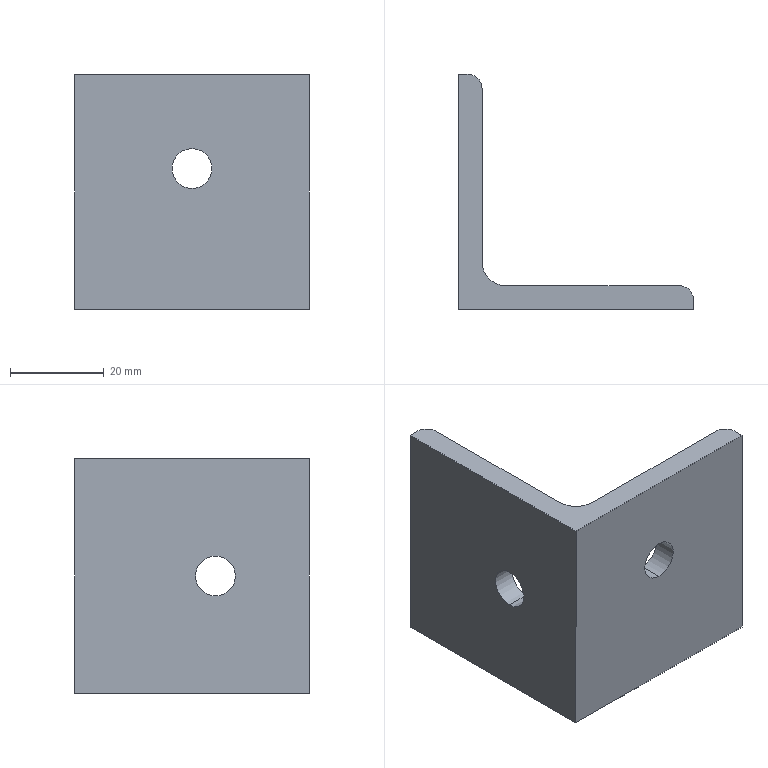Part | STEP file | 750038244 | 1 solid | 15 faces | box 50 x 50 x 50 mm | volume 23258 mm3 | plane 8 | cylinder 7 | commonest cylinder face diameters 8.5 x4 6 x2 10 x1
STEP:
#1=CARTESIAN_POINT('',(5.,20.,20.75));
#2=VERTEX_POINT('',#1);
#3=CARTESIAN_POINT('',(5.,20.,29.25));
#4=VERTEX_POINT('',#3);
#5=CARTESIAN_POINT('',(5.,20.,25.));
#6=DIRECTION('',(-1.,0.,0.));
#7=DIRECTION('',(0.,0.,1.));
#8=AXIS2_PLACEMENT_3D('',#5,#6,#7);
#9=CIRCLE('',#8,4.25);
#10=EDGE_CURVE('',#2,#4,#9,.T.);
#11=ORIENTED_EDGE('',*,*,#10,.F.);
#12=CARTESIAN_POINT('',(0.,20.,20.75));
#13=VERTEX_POINT('',#12);
#14=CARTESIAN_POINT('',(55.,20.,20.75));
#15=DIRECTION('',(-1.,0.,0.));
#16=VECTOR('',#15,1000.);
#17=LINE('',#14,#16);
#18=EDGE_CURVE('',#2,#13,#17,.T.);
#19=ORIENTED_EDGE('',*,*,#18,.T.);
#20=CARTESIAN_POINT('',(0.,20.,29.25));
#21=VERTEX_POINT('',#20);
#22=CARTESIAN_POINT('',(0.,20.,25.));
#23=DIRECTION('',(-1.,0.,0.));
#24=DIRECTION('',(0.,0.,1.));
#25=AXIS2_PLACEMENT_3D('',#22,#23,#24);
#26=CIRCLE('',#25,4.25);
#27=EDGE_CURVE('',#13,#21,#26,.T.);
#28=ORIENTED_EDGE('',*,*,#27,.T.);
#29=CARTESIAN_POINT('',(55.,20.,29.25));
#30=DIRECTION('',(-1.,0.,0.));
#31=VECTOR('',#30,1000.);
#32=LINE('',#29,#31);
#33=EDGE_CURVE('',#4,#21,#32,.T.);
#34=ORIENTED_EDGE('',*,*,#33,.F.);
#35=EDGE_LOOP('',(#11,#19,#28,#34));
#36=FACE_OUTER_BOUND('',#35,.T.);
#37=CARTESIAN_POINT('',(55.,20.,25.));
#38=DIRECTION('',(-1.,0.,0.));
#39=DIRECTION('',(0.,0.,1.));
#40=AXIS2_PLACEMENT_3D('',#37,#38,#39);
#41=CYLINDRICAL_SURFACE('',#40,4.25);
#42=ADVANCED_FACE('',(#36),#41,.F.);
#43=CARTESIAN_POINT('',(25.,5.,25.75));
#44=VERTEX_POINT('',#43);
#45=CARTESIAN_POINT('',(25.,5.,34.25));
#46=VERTEX_POINT('',#45);
#47=CARTESIAN_POINT('',(25.,5.,30.));
#48=DIRECTION('',(0.,1.,0.));
#49=DIRECTION('',(0.,0.,-1.));
#50=AXIS2_PLACEMENT_3D('',#47,#48,#49);
#51=CIRCLE('',#50,4.25);
#52=EDGE_CURVE('',#44,#46,#51,.T.);
#53=ORIENTED_EDGE('',*,*,#52,.T.);
#54=CARTESIAN_POINT('',(25.,0.,34.25));
#55=VERTEX_POINT('',#54);
#56=CARTESIAN_POINT('',(25.,55.,34.25));
#57=DIRECTION('',(0.,-1.,0.));
#58=VECTOR('',#57,1000.);
#59=LINE('',#56,#58);
#60=EDGE_CURVE('',#46,#55,#59,.T.);
#61=ORIENTED_EDGE('',*,*,#60,.T.);
#62=CARTESIAN_POINT('',(25.,0.,25.75));
#63=VERTEX_POINT('',#62);
#64=CARTESIAN_POINT('',(25.,0.,30.));
#65=DIRECTION('',(0.,-1.,0.));
#66=DIRECTION('',(0.,0.,-1.));
#67=AXIS2_PLACEMENT_3D('',#64,#65,#66);
#68=CIRCLE('',#67,4.25);
#69=EDGE_CURVE('',#55,#63,#68,.T.);
#70=ORIENTED_EDGE('',*,*,#69,.T.);
#71=CARTESIAN_POINT('',(25.,55.,25.75));
#72=DIRECTION('',(0.,-1.,0.));
#73=VECTOR('',#72,1000.);
#74=LINE('',#71,#73);
#75=EDGE_CURVE('',#44,#63,#74,.T.);
#76=ORIENTED_EDGE('',*,*,#75,.F.);
#77=EDGE_LOOP('',(#53,#61,#70,#76));
#78=FACE_OUTER_BOUND('',#77,.T.);
#79=CARTESIAN_POINT('',(25.,55.,30.));
#80=DIRECTION('',(0.,-1.,0.));
#81=DIRECTION('',(0.,0.,-1.));
#82=AXIS2_PLACEMENT_3D('',#79,#80,#81);
#83=CYLINDRICAL_SURFACE('',#82,4.25);
#84=ADVANCED_FACE('',(#78),#83,.F.);
#85=CARTESIAN_POINT('',(0.,0.,50.));
#86=VERTEX_POINT('',#85);
#87=CARTESIAN_POINT('',(0.,0.,0.));
#88=VERTEX_POINT('',#87);
#89=CARTESIAN_POINT('',(0.,0.,50.));
#90=DIRECTION('',(0.,0.,-1.));
#91=VECTOR('',#90,1000.);
#92=LINE('',#89,#91);
#93=EDGE_CURVE('',#86,#88,#92,.T.);
#94=ORIENTED_EDGE('',*,*,#93,.F.);
#95=CARTESIAN_POINT('',(0.,50.,50.));
#96=VERTEX_POINT('',#95);
#97=CARTESIAN_POINT('',(0.,50.,50.));
#98=DIRECTION('',(0.,-1.,0.));
#99=VECTOR('',#98,1000.);
#100=LINE('',#97,#99);
#101=EDGE_CURVE('',#96,#86,#100,.T.);
#102=ORIENTED_EDGE('',*,*,#101,.F.);
#103=CARTESIAN_POINT('',(0.,50.,0.));
#104=VERTEX_POINT('',#103);
#105=CARTESIAN_POINT('',(0.,50.,50.));
#106=DIRECTION('',(0.,0.,1.));
#107=VECTOR('',#106,1000.);
#108=LINE('',#105,#107);
#109=EDGE_CURVE('',#104,#96,#108,.T.);
#110=ORIENTED_EDGE('',*,*,#109,.F.);
#111=CARTESIAN_POINT('',(0.,50.,0.));
#112=DIRECTION('',(0.,1.,0.));
#113=VECTOR('',#112,1000.);
#114=LINE('',#111,#113);
#115=EDGE_CURVE('',#88,#104,#114,.T.);
#116=ORIENTED_EDGE('',*,*,#115,.F.);
#117=EDGE_LOOP('',(#94,#102,#110,#116));
#118=FACE_OUTER_BOUND('',#117,.T.);
#119=CARTESIAN_POINT('',(0.,20.,25.));
#120=DIRECTION('',(-1.,0.,0.));
#121=DIRECTION('',(0.,0.,1.));
#122=AXIS2_PLACEMENT_3D('',#119,#120,#121);
#123=CIRCLE('',#122,4.25);
#124=EDGE_CURVE('',#21,#13,#123,.T.);
#125=ORIENTED_EDGE('',*,*,#124,.F.);
#126=ORIENTED_EDGE('',*,*,#27,.F.);
#127=EDGE_LOOP('',(#125,#126));
#128=FACE_BOUND('',#127,.T.);
#129=CARTESIAN_POINT('',(0.,50.,50.));
#130=DIRECTION('',(1.,0.,0.));
#131=DIRECTION('',(0.,1.,0.));
#132=AXIS2_PLACEMENT_3D('',#129,#130,#131);
#133=PLANE('',#132);
#134=ADVANCED_FACE('',(#118,#128),#133,.F.);
#135=CARTESIAN_POINT('',(2.,50.,0.));
#136=VERTEX_POINT('',#135);
#137=CARTESIAN_POINT('',(47.,50.,0.));
#138=DIRECTION('',(-1.,0.,0.));
#139=VECTOR('',#138,1000.);
#140=LINE('',#137,#139);
#141=EDGE_CURVE('',#136,#104,#140,.T.);
#142=ORIENTED_EDGE('',*,*,#141,.F.);
#143=CARTESIAN_POINT('',(5.,47.,0.));
#144=VERTEX_POINT('',#143);
#145=CARTESIAN_POINT('',(2.,47.,0.));
#146=DIRECTION('',(0.,0.,1.));
#147=DIRECTION('',(-1.,0.,0.));
#148=AXIS2_PLACEMENT_3D('',#145,#146,#147);
#149=CIRCLE('',#148,3.);
#150=EDGE_CURVE('',#144,#136,#149,.T.);
#151=ORIENTED_EDGE('',*,*,#150,.F.);
#152=CARTESIAN_POINT('',(5.,10.,0.));
#153=VERTEX_POINT('',#152);
#154=CARTESIAN_POINT('',(5.,2.,0.));
#155=DIRECTION('',(0.,1.,0.));
#156=VECTOR('',#155,1000.);
#157=LINE('',#154,#156);
#158=EDGE_CURVE('',#153,#144,#157,.T.);
#159=ORIENTED_EDGE('',*,*,#158,.F.);
#160=CARTESIAN_POINT('',(10.,5.,0.));
#161=VERTEX_POINT('',#160);
#162=CARTESIAN_POINT('',(10.,10.,0.));
#163=DIRECTION('',(0.,0.,-1.));
#164=DIRECTION('',(-1.,0.,0.));
#165=AXIS2_PLACEMENT_3D('',#162,#163,#164);
#166=CIRCLE('',#165,5.);
#167=EDGE_CURVE('',#161,#153,#166,.T.);
#168=ORIENTED_EDGE('',*,*,#167,.F.);
#169=CARTESIAN_POINT('',(47.,5.,0.));
#170=VERTEX_POINT('',#169);
#171=CARTESIAN_POINT('',(47.,5.,0.));
#172=DIRECTION('',(-1.,0.,0.));
#173=VECTOR('',#172,1000.);
#174=LINE('',#171,#173);
#175=EDGE_CURVE('',#170,#161,#174,.T.);
#176=ORIENTED_EDGE('',*,*,#175,.F.);
#177=CARTESIAN_POINT('',(50.,2.,0.));
#178=VERTEX_POINT('',#177);
#179=CARTESIAN_POINT('',(47.,2.,0.));
#180=DIRECTION('',(0.,0.,1.));
#181=DIRECTION('',(-1.,0.,0.));
#182=AXIS2_PLACEMENT_3D('',#179,#180,#181);
#183=CIRCLE('',#182,3.);
#184=EDGE_CURVE('',#178,#170,#183,.T.);
#185=ORIENTED_EDGE('',*,*,#184,.F.);
#186=CARTESIAN_POINT('',(50.,0.,0.));
#187=VERTEX_POINT('',#186);
#188=CARTESIAN_POINT('',(50.,2.,0.));
#189=DIRECTION('',(0.,1.,0.));
#190=VECTOR('',#189,1000.);
#191=LINE('',#188,#190);
#192=EDGE_CURVE('',#187,#178,#191,.T.);
#193=ORIENTED_EDGE('',*,*,#192,.F.);
#194=CARTESIAN_POINT('',(47.,0.,0.));
#195=DIRECTION('',(1.,0.,0.));
#196=VECTOR('',#195,1000.);
#197=LINE('',#194,#196);
#198=EDGE_CURVE('',#88,#187,#197,.T.);
#199=ORIENTED_EDGE('',*,*,#198,.F.);
#200=ORIENTED_EDGE('',*,*,#115,.T.);
#201=EDGE_LOOP('',(#142,#151,#159,#168,#176,#185,#193,#199,#200));
#202=FACE_OUTER_BOUND('',#201,.T.);
#203=CARTESIAN_POINT('',(47.,2.,0.));
#204=DIRECTION('',(0.,0.,1.));
#205=DIRECTION('',(1.,0.,0.));
#206=AXIS2_PLACEMENT_3D('',#203,#204,#205);
#207=PLANE('',#206);
#208=ADVANCED_FACE('',(#202),#207,.F.);
#209=CARTESIAN_POINT('',(50.,0.,50.));
#210=VERTEX_POINT('',#209);
#211=CARTESIAN_POINT('',(50.,0.,50.));
#212=DIRECTION('',(0.,0.,-1.));
#213=VECTOR('',#212,1000.);
#214=LINE('',#211,#213);
#215=EDGE_CURVE('',#210,#187,#214,.T.);
#216=ORIENTED_EDGE('',*,*,#215,.F.);
#217=CARTESIAN_POINT('',(0.,0.,50.));
#218=DIRECTION('',(1.,0.,0.));
#219=VECTOR('',#218,1000.);
#220=LINE('',#217,#219);
#221=EDGE_CURVE('',#86,#210,#220,.T.);
#222=ORIENTED_EDGE('',*,*,#221,.F.);
#223=ORIENTED_EDGE('',*,*,#93,.T.);
#224=ORIENTED_EDGE('',*,*,#198,.T.);
#225=EDGE_LOOP('',(#216,#222,#223,#224));
#226=FACE_OUTER_BOUND('',#225,.T.);
#227=CARTESIAN_POINT('',(25.,0.,30.));
#228=DIRECTION('',(0.,-1.,0.));
#229=DIRECTION('',(0.,0.,-1.));
#230=AXIS2_PLACEMENT_3D('',#227,#228,#229);
#231=CIRCLE('',#230,4.25);
#232=EDGE_CURVE('',#63,#55,#231,.T.);
#233=ORIENTED_EDGE('',*,*,#232,.F.);
#234=ORIENTED_EDGE('',*,*,#69,.F.);
#235=EDGE_LOOP('',(#233,#234));
#236=FACE_BOUND('',#235,.T.);
#237=CARTESIAN_POINT('',(0.,0.,50.));
#238=DIRECTION('',(0.,1.,0.));
#239=DIRECTION('',(0.,0.,1.));
#240=AXIS2_PLACEMENT_3D('',#237,#238,#239);
#241=PLANE('',#240);
#242=ADVANCED_FACE('',(#226,#236),#241,.F.);
#243=CARTESIAN_POINT('',(5.,47.,50.));
#244=VERTEX_POINT('',#243);
#245=CARTESIAN_POINT('',(2.,50.,50.));
#246=VERTEX_POINT('',#245);
#247=CARTESIAN_POINT('',(2.,47.,50.));
#248=DIRECTION('',(0.,0.,1.));
#249=DIRECTION('',(-1.,0.,0.));
#250=AXIS2_PLACEMENT_3D('',#247,#248,#249);
#251=CIRCLE('',#250,3.);
#252=EDGE_CURVE('',#244,#246,#251,.T.);
#253=ORIENTED_EDGE('',*,*,#252,.T.);
#254=CARTESIAN_POINT('',(47.,50.,50.));
#255=DIRECTION('',(-1.,0.,0.));
#256=VECTOR('',#255,1000.);
#257=LINE('',#254,#256);
#258=EDGE_CURVE('',#246,#96,#257,.T.);
#259=ORIENTED_EDGE('',*,*,#258,.T.);
#260=ORIENTED_EDGE('',*,*,#101,.T.);
#261=ORIENTED_EDGE('',*,*,#221,.T.);
#262=CARTESIAN_POINT('',(50.,2.,50.));
#263=VERTEX_POINT('',#262);
#264=CARTESIAN_POINT('',(50.,2.,50.));
#265=DIRECTION('',(0.,1.,0.));
#266=VECTOR('',#265,1000.);
#267=LINE('',#264,#266);
#268=EDGE_CURVE('',#210,#263,#267,.T.);
#269=ORIENTED_EDGE('',*,*,#268,.T.);
#270=CARTESIAN_POINT('',(47.,5.,50.));
#271=VERTEX_POINT('',#270);
#272=CARTESIAN_POINT('',(47.,2.,50.));
#273=DIRECTION('',(0.,0.,1.));
#274=DIRECTION('',(-1.,0.,0.));
#275=AXIS2_PLACEMENT_3D('',#272,#273,#274);
#276=CIRCLE('',#275,3.);
#277=EDGE_CURVE('',#263,#271,#276,.T.);
#278=ORIENTED_EDGE('',*,*,#277,.T.);
#279=CARTESIAN_POINT('',(10.,5.,50.));
#280=VERTEX_POINT('',#279);
#281=CARTESIAN_POINT('',(47.,5.,50.));
#282=DIRECTION('',(-1.,0.,0.));
#283=VECTOR('',#282,1000.);
#284=LINE('',#281,#283);
#285=EDGE_CURVE('',#271,#280,#284,.T.);
#286=ORIENTED_EDGE('',*,*,#285,.T.);
#287=CARTESIAN_POINT('',(5.,10.,50.));
#288=VERTEX_POINT('',#287);
#289=CARTESIAN_POINT('',(10.,10.,50.));
#290=DIRECTION('',(0.,0.,-1.));
#291=DIRECTION('',(-1.,0.,0.));
#292=AXIS2_PLACEMENT_3D('',#289,#290,#291);
#293=CIRCLE('',#292,5.);
#294=EDGE_CURVE('',#280,#288,#293,.T.);
#295=ORIENTED_EDGE('',*,*,#294,.T.);
#296=CARTESIAN_POINT('',(5.,2.,50.));
#297=DIRECTION('',(0.,1.,0.));
#298=VECTOR('',#297,1000.);
#299=LINE('',#296,#298);
#300=EDGE_CURVE('',#288,#244,#299,.T.);
#301=ORIENTED_EDGE('',*,*,#300,.T.);
#302=EDGE_LOOP('',(#253,#259,#260,#261,#269,#278,#286,#295,#301));
#303=FACE_OUTER_BOUND('',#302,.T.);
#304=CARTESIAN_POINT('',(47.,2.,50.));
#305=DIRECTION('',(0.,0.,1.));
#306=DIRECTION('',(1.,0.,0.));
#307=AXIS2_PLACEMENT_3D('',#304,#305,#306);
#308=PLANE('',#307);
#309=ADVANCED_FACE('',(#303),#308,.T.);
#310=ORIENTED_EDGE('',*,*,#109,.T.);
#311=ORIENTED_EDGE('',*,*,#258,.F.);
#312=CARTESIAN_POINT('',(2.,50.,50.));
#313=DIRECTION('',(0.,0.,1.));
#314=VECTOR('',#313,1000.);
#315=LINE('',#312,#314);
#316=EDGE_CURVE('',#136,#246,#315,.T.);
#317=ORIENTED_EDGE('',*,*,#316,.F.);
#318=ORIENTED_EDGE('',*,*,#141,.T.);
#319=EDGE_LOOP('',(#310,#311,#317,#318));
#320=FACE_OUTER_BOUND('',#319,.T.);
#321=CARTESIAN_POINT('',(2.,50.,50.));
#322=DIRECTION('',(0.,-1.,0.));
#323=DIRECTION('',(0.,0.,-1.));
#324=AXIS2_PLACEMENT_3D('',#321,#322,#323);
#325=PLANE('',#324);
#326=ADVANCED_FACE('',(#320),#325,.F.);
#327=ORIENTED_EDGE('',*,*,#18,.F.);
#328=CARTESIAN_POINT('',(5.,20.,25.));
#329=DIRECTION('',(-1.,0.,0.));
#330=DIRECTION('',(0.,0.,1.));
#331=AXIS2_PLACEMENT_3D('',#328,#329,#330);
#332=CIRCLE('',#331,4.25);
#333=EDGE_CURVE('',#4,#2,#332,.T.);
#334=ORIENTED_EDGE('',*,*,#333,.F.);
#335=ORIENTED_EDGE('',*,*,#33,.T.);
#336=ORIENTED_EDGE('',*,*,#124,.T.);
#337=EDGE_LOOP('',(#327,#334,#335,#336));
#338=FACE_OUTER_BOUND('',#337,.T.);
#339=CARTESIAN_POINT('',(55.,20.,25.));
#340=DIRECTION('',(-1.,0.,0.));
#341=DIRECTION('',(0.,0.,1.));
#342=AXIS2_PLACEMENT_3D('',#339,#340,#341);
#343=CYLINDRICAL_SURFACE('',#342,4.25);
#344=ADVANCED_FACE('',(#338),#343,.F.);
#345=ORIENTED_EDGE('',*,*,#252,.F.);
#346=CARTESIAN_POINT('',(5.,47.,50.));
#347=DIRECTION('',(0.,0.,-1.));
#348=VECTOR('',#347,1000.);
#349=LINE('',#346,#348);
#350=EDGE_CURVE('',#244,#144,#349,.T.);
#351=ORIENTED_EDGE('',*,*,#350,.T.);
#352=ORIENTED_EDGE('',*,*,#150,.T.);
#353=ORIENTED_EDGE('',*,*,#316,.T.);
#354=EDGE_LOOP('',(#345,#351,#352,#353));
#355=FACE_OUTER_BOUND('',#354,.T.);
#356=CARTESIAN_POINT('',(2.,47.,50.));
#357=DIRECTION('',(0.,0.,-1.));
#358=DIRECTION('',(-1.,0.,0.));
#359=AXIS2_PLACEMENT_3D('',#356,#357,#358);
#360=CYLINDRICAL_SURFACE('',#359,3.);
#361=ADVANCED_FACE('',(#355),#360,.T.);
#362=ORIENTED_EDGE('',*,*,#350,.F.);
#363=ORIENTED_EDGE('',*,*,#300,.F.);
#364=CARTESIAN_POINT('',(5.,10.,50.));
#365=DIRECTION('',(0.,0.,1.));
#366=VECTOR('',#365,1000.);
#367=LINE('',#364,#366);
#368=EDGE_CURVE('',#153,#288,#367,.T.);
#369=ORIENTED_EDGE('',*,*,#368,.F.);
#370=ORIENTED_EDGE('',*,*,#158,.T.);
#371=EDGE_LOOP('',(#362,#363,#369,#370));
#372=FACE_OUTER_BOUND('',#371,.T.);
#373=ORIENTED_EDGE('',*,*,#333,.T.);
#374=ORIENTED_EDGE('',*,*,#10,.T.);
#375=EDGE_LOOP('',(#373,#374));
#376=FACE_BOUND('',#375,.T.);
#377=CARTESIAN_POINT('',(5.,10.,50.));
#378=DIRECTION('',(-1.,0.,0.));
#379=DIRECTION('',(0.,-1.,0.));
#380=AXIS2_PLACEMENT_3D('',#377,#378,#379);
#381=PLANE('',#380);
#382=ADVANCED_FACE('',(#372,#376),#381,.F.);
#383=ORIENTED_EDGE('',*,*,#368,.T.);
#384=ORIENTED_EDGE('',*,*,#294,.F.);
#385=CARTESIAN_POINT('',(10.,5.,50.));
#386=DIRECTION('',(0.,0.,1.));
#387=VECTOR('',#386,1000.);
#388=LINE('',#385,#387);
#389=EDGE_CURVE('',#161,#280,#388,.T.);
#390=ORIENTED_EDGE('',*,*,#389,.F.);
#391=ORIENTED_EDGE('',*,*,#167,.T.);
#392=EDGE_LOOP('',(#383,#384,#390,#391));
#393=FACE_OUTER_BOUND('',#392,.T.);
#394=CARTESIAN_POINT('',(10.,10.,50.));
#395=DIRECTION('',(0.,0.,-1.));
#396=DIRECTION('',(-1.,0.,0.));
#397=AXIS2_PLACEMENT_3D('',#394,#395,#396);
#398=CYLINDRICAL_SURFACE('',#397,5.);
#399=ADVANCED_FACE('',(#393),#398,.F.);
#400=ORIENTED_EDGE('',*,*,#389,.T.);
#401=ORIENTED_EDGE('',*,*,#285,.F.);
#402=CARTESIAN_POINT('',(47.,5.,50.));
#403=DIRECTION('',(0.,0.,1.));
#404=VECTOR('',#403,1000.);
#405=LINE('',#402,#404);
#406=EDGE_CURVE('',#170,#271,#405,.T.);
#407=ORIENTED_EDGE('',*,*,#406,.F.);
#408=ORIENTED_EDGE('',*,*,#175,.T.);
#409=EDGE_LOOP('',(#400,#401,#407,#408));
#410=FACE_OUTER_BOUND('',#409,.T.);
#411=ORIENTED_EDGE('',*,*,#52,.F.);
#412=CARTESIAN_POINT('',(25.,5.,30.));
#413=DIRECTION('',(0.,1.,0.));
#414=DIRECTION('',(0.,0.,-1.));
#415=AXIS2_PLACEMENT_3D('',#412,#413,#414);
#416=CIRCLE('',#415,4.25);
#417=EDGE_CURVE('',#46,#44,#416,.T.);
#418=ORIENTED_EDGE('',*,*,#417,.F.);
#419=EDGE_LOOP('',(#411,#418));
#420=FACE_BOUND('',#419,.T.);
#421=CARTESIAN_POINT('',(47.,5.,50.));
#422=DIRECTION('',(0.,-1.,0.));
#423=DIRECTION('',(0.,0.,-1.));
#424=AXIS2_PLACEMENT_3D('',#421,#422,#423);
#425=PLANE('',#424);
#426=ADVANCED_FACE('',(#410,#420),#425,.F.);
#427=ORIENTED_EDGE('',*,*,#277,.F.);
#428=CARTESIAN_POINT('',(50.,2.,50.));
#429=DIRECTION('',(0.,0.,-1.));
#430=VECTOR('',#429,1000.);
#431=LINE('',#428,#430);
#432=EDGE_CURVE('',#263,#178,#431,.T.);
#433=ORIENTED_EDGE('',*,*,#432,.T.);
#434=ORIENTED_EDGE('',*,*,#184,.T.);
#435=ORIENTED_EDGE('',*,*,#406,.T.);
#436=EDGE_LOOP('',(#427,#433,#434,#435));
#437=FACE_OUTER_BOUND('',#436,.T.);
#438=CARTESIAN_POINT('',(47.,2.,50.));
#439=DIRECTION('',(0.,0.,-1.));
#440=DIRECTION('',(-1.,0.,0.));
#441=AXIS2_PLACEMENT_3D('',#438,#439,#440);
#442=CYLINDRICAL_SURFACE('',#441,3.);
#443=ADVANCED_FACE('',(#437),#442,.T.);
#444=ORIENTED_EDGE('',*,*,#432,.F.);
#445=ORIENTED_EDGE('',*,*,#268,.F.);
#446=ORIENTED_EDGE('',*,*,#215,.T.);
#447=ORIENTED_EDGE('',*,*,#192,.T.);
#448=EDGE_LOOP('',(#444,#445,#446,#447));
#449=FACE_OUTER_BOUND('',#448,.T.);
#450=CARTESIAN_POINT('',(50.,0.,50.));
#451=DIRECTION('',(-1.,0.,0.));
#452=DIRECTION('',(0.,0.,1.));
#453=AXIS2_PLACEMENT_3D('',#450,#451,#452);
#454=PLANE('',#453);
#455=ADVANCED_FACE('',(#449),#454,.F.);
#456=ORIENTED_EDGE('',*,*,#60,.F.);
#457=ORIENTED_EDGE('',*,*,#417,.T.);
#458=ORIENTED_EDGE('',*,*,#75,.T.);
#459=ORIENTED_EDGE('',*,*,#232,.T.);
#460=EDGE_LOOP('',(#456,#457,#458,#459));
#461=FACE_OUTER_BOUND('',#460,.T.);
#462=CARTESIAN_POINT('',(25.,55.,30.));
#463=DIRECTION('',(0.,-1.,0.));
#464=DIRECTION('',(0.,0.,-1.));
#465=AXIS2_PLACEMENT_3D('',#462,#463,#464);
#466=CYLINDRICAL_SURFACE('',#465,4.25);
#467=ADVANCED_FACE('',(#461),#466,.F.);
#468=CLOSED_SHELL('',(#42,#84,#134,#208,#242,#309,#326,#344,#361,#382,#399,#426,#443,#455,#467));
#469=MANIFOLD_SOLID_BREP('',#468);
#470=CARTESIAN_POINT('',(0.,0.,0.));
#471=DIRECTION('',(0.,0.,1.));
#472=DIRECTION('',(1.,0.,0.));
#473=AXIS2_PLACEMENT_3D('',#470,#471,#472);
#474=(LENGTH_UNIT()NAMED_UNIT(*)SI_UNIT(.MILLI.,.METRE.));
#475=UNCERTAINTY_MEASURE_WITH_UNIT(LENGTH_MEASURE(0.00001),#474,'','');
#476=(NAMED_UNIT(*)PLANE_ANGLE_UNIT()SI_UNIT($,.RADIAN.));
#477=(NAMED_UNIT(*)SI_UNIT($,.STERADIAN.)SOLID_ANGLE_UNIT());
#478=(GEOMETRIC_REPRESENTATION_CONTEXT(3)GLOBAL_UNCERTAINTY_ASSIGNED_CONTEXT((#475))GLOBAL_UNIT_ASSIGNED_CONTEXT((#474,#476,#477))REPRESENTATION_CONTEXT('',''));
#479=ADVANCED_BREP_SHAPE_REPRESENTATION('',(#469,#473),#478);